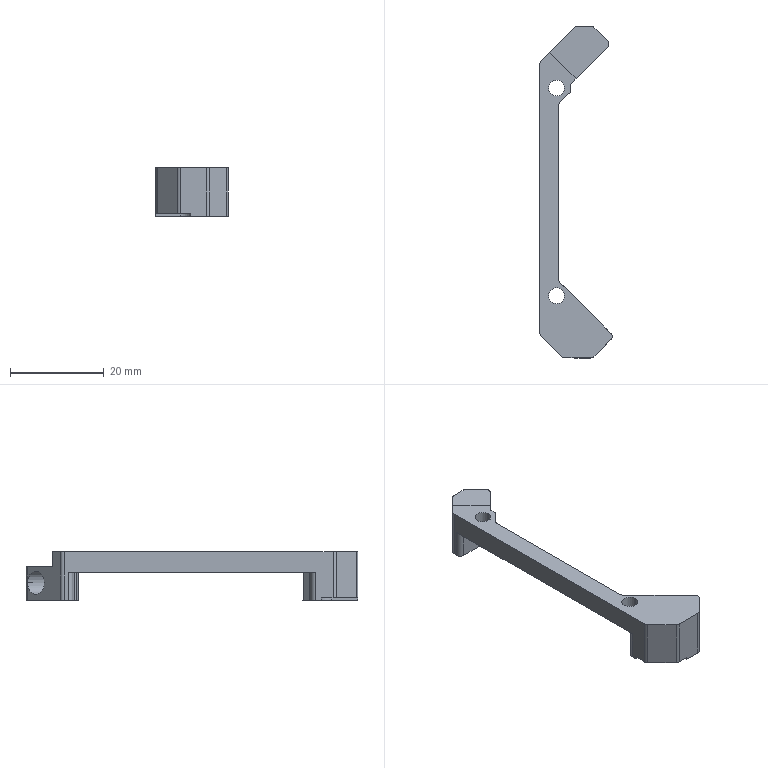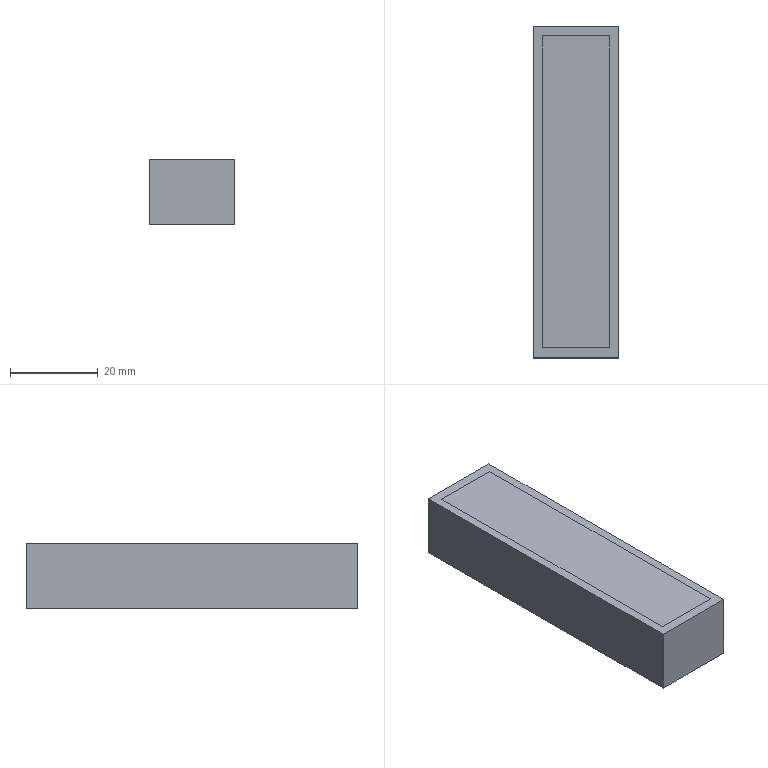CAM job | NX | 3+2 milling, drilling | part box 15.463 x 71 x 10.4 mm | stock box 19.463 x 75.537 x 15 mm
Tools:
number,name,description,diameter,corner_radius,flute_length,length,flutes
5,D4点钻,定心钻D4,4.0,0.0,43.0,75.0,2
3,D2-ROUGHING,D2,2.0,0.0,6.0,50.0,2
11,D3-ROUGHING,D3,3.0,0.0,9.0,50.0,2
7,D4-FINISHING,D4,4.0,0.0,12.0,50.0,2
2,D8-ROUGHING,D8,8.0,0.0,20.0,60.0,2
4,D8-FINISHING,D8,8.0,0.0,20.0,60.0,2
5,D4倒角刀,DJ4-32,4.0,0.0,2.0,50.0,2
1,D54-面刀,Milling Tool-5 Parameters,50.0,0.0,50.0,75.0,2
6,DRILL-3.4,Drilling Tool,3.4,0.0,35.0,50.0,2
10,DRILL-3,Drilling Tool,3.0,0.0,35.0,50.0,2
Operations:
program,operation,operation_type,tool,method,geometry_group,spindle_rpm,surface_speed,feed_per_tooth,feed_cut,feed_plunge,cut_length_mm,path_length_mm,cut_time_min,machine_time_min
G54,FLOOR_FACING,VolumeBased25DMillingOperation,D54-面刀,METHOD,W1,4500.0,706.0,0.0556,500.0,100.0,137.0,231.0,0.274,0.2834
G54,ADAPTIVE_MILLING,CavityMilling,D8-ROUGHING,METHOD,W1,5000.0,125.0,0.3,3000.0,100.0,1565.868,1857.268,0.3669,0.396
G54,PLANAR_MILL_1,PlanarMilling,D2-ROUGHING,METHOD,W1,4000.0,25.0,0.1,800.0,100.0,99.648,254.928,0.1246,0.1401
G54,PLANAR_MILL_1_COPY_1,PlanarMilling,D2-ROUGHING,METHOD,W1,4000.0,25.0,0.1,800.0,100.0,52.68,178.33,0.0658,0.0784
G54,PLANAR_MILL_1_COPY,PlanarMilling,D2-ROUGHING,METHOD,W1,4000.0,25.0,0.0187,150.0,100.0,60.303,257.049,0.402,0.4217
G54,PLANAR_MILL,PlanarMilling,D8-FINISHING,METHOD,W1,5000.0,125.0,0.07,700.0,100.0,424.698,542.698,0.6067,0.6185
G54,PLANAR_MILL_COPY,PlanarMilling,D8-FINISHING,METHOD,W1,5000.0,125.0,0.07,700.0,100.0,48.0,267.682,0.0686,0.0905
G54,PECK_DRILLING,Operation,D4点钻,METHOD,W1,2500.0,18.0,0.05,150.0,0.0,9.4,166.321,0.0627,0.0784
G54,PLANAR_MILL_2,PlanarMilling,D4点钻,METHOD,W1,3000.0,37.0,0.1333,800.0,100.0,169.216,266.216,0.2115,0.2212
G54,PLANAR_MILL_2_COPY,PlanarMilling,D4点钻,METHOD,W1,3000.0,37.0,0.1333,800.0,100.0,37.774,141.274,0.0472,0.0576
G54,PECK_DRILLING_COPY,Operation,DRILL-3.4,METHOD,W1,2500.0,26.0,0.02,100.0,0.0,22.0,191.521,0.22,0.237
G55,FLOOR_FACING_1,VolumeBased25DMillingOperation,D54-面刀,METHOD,W2,4500.0,706.0,0.2222,2000.0,100.0,665.0,1672.4,0.3325,0.4332
G55,FLOOR_FACING_1_COPY,VolumeBased25DMillingOperation,D54-面刀,METHOD,W2,4500.0,706.0,0.0556,500.0,100.0,133.0,237.0,0.266,0.2764
G55,CAVITY_MILL,CavityMilling,D8-ROUGHING,METHOD,W2,5000.0,125.0,0.25,2500.0,100.0,659.673,1089.973,0.2639,0.3069
G55,PLANAR_MILL_3,PlanarMilling,D2-ROUGHING,METHOD,W2,4500.0,28.0,0.1111,1000.0,100.0,156.349,385.613,0.1563,0.1793
G55,PLANAR_MILL_3_COPY,PlanarMilling,D2-ROUGHING,METHOD,W2,4500.0,28.0,0.0333,300.0,100.0,105.891,331.775,0.353,0.3756
G55,PLANAR_MILL_4,PlanarMilling,D8-FINISHING,METHOD,W2,4500.0,113.0,0.0778,700.0,100.0,70.096,317.964,0.1001,0.1249
G55,PLANAR_MILL_4_COPY,PlanarMilling,D8-FINISHING,METHOD,W2,4500.0,113.0,0.0778,700.0,100.0,58.079,164.079,0.083,0.0936
G55,PLANAR_MILL_4_COPY_COPY,PlanarMilling,D4-FINISHING,METHOD,W2,4500.0,56.0,0.1111,1000.0,100.0,31.456,127.456,0.0315,0.0411
G55,PLANAR_MILL_4_COPY_COPY_COPY,PlanarMilling,D4-FINISHING,METHOD,W2,4500.0,56.0,0.0556,500.0,100.0,32.495,128.495,0.065,0.0746
G55,SPOT_DRILLING,Operation,D4倒角刀,METHOD,W2,1500.0,18.0,0.05,150.0,0.0,9.4,69.321,0.0627,0.0687
G55,PLANAR_MILL_5,PlanarMilling,D4倒角刀,METHOD,W2,4500.0,56.0,0.1111,1000.0,100.0,59.426,154.326,0.0594,0.0689
G55,PLANAR_MILL_5_COPY_1,PlanarMilling,D4倒角刀,METHOD,W2,4500.0,56.0,0.1111,1000.0,100.0,20.772,117.772,0.0208,0.0305
G55,PLANAR_MILL_5_COPY,PlanarMilling,D4倒角刀,METHOD,W2,4500.0,56.0,0.1111,1000.0,100.0,57.074,153.073,0.0571,0.0667
G55,PLANAR_MILL_5_COPY_COPY,PlanarMilling,D4倒角刀,METHOD,W2,4500.0,56.0,0.1111,1000.0,100.0,112.25,340.907,0.1123,0.1351
钳口-虎钳,SPOT_DRILLING_1,Operation,D4倒角刀,METHOD,虎钳-钳口,1500.0,18.0,0.05,150.0,0.0,40.5,250.359,0.27,0.291
钳口-虎钳,SPOT_DRILLING_1_COPY,Operation,DRILL-3,METHOD,虎钳-钳口,1500.0,18.0,0.05,150.0,0.0,81.0,331.359,0.54,0.565
钳口-虎钳,FLOOR_WALL,VolumeBased25DMillingOperation,D3-ROUGHING,METHOD,虎钳-钳口,5000.0,47.0,0.2,2000.0,100.0,1956.725,2277.783,0.9784,1.01
钳口-虎钳,FLOOR_WALL_COPY_COPY,VolumeBased25DMillingOperation,D2-ROUGHING,METHOD,虎钳-钳口,5000.0,31.0,0.08,800.0,100.0,341.296,421.147,0.4266,0.4346
钳口-虎钳,FLOOR_WALL_COPY,VolumeBased25DMillingOperation,D2-ROUGHING,METHOD,虎钳-钳口,5000.0,31.0,0.08,800.0,100.0,355.509,401.309,0.4444,0.449
钳口-虎钳,FLOOR_WALL_COPY_COPY_COPY,VolumeBased25DMillingOperation,D2-ROUGHING,METHOD,虎钳-钳口,5000.0,31.0,0.08,800.0,100.0,170.748,211.538,0.2134,0.2175
氧化后加工,FLOOR_WALL_1,VolumeBased25DMillingOperation,D4-FINISHING,METHOD,MCS_3,4000.0,50.0,0.1,800.0,100.0,198.584,325.005,0.2482,0.2609
氧化后加工,PLANAR_MILL_6,PlanarMilling,D4-FINISHING,METHOD,MCS_3,4000.0,50.0,0.025,200.0,100.0,9.712,121.112,0.0486,0.0597
氧化后加工,PLANAR_MILL_6_COPY,PlanarMilling,D4-FINISHING,METHOD,MCS_3,4000.0,50.0,0.025,200.0,100.0,24.74,130.84,0.1237,0.1343
氧化后加工,PLANAR_MILL_7,PlanarMilling,D4点钻,METHOD,MCS_3,3000.0,37.0,0.1167,700.0,100.0,22.336,119.336,0.0319,0.0416
氧化后加工,PLANAR_MILL_7_COPY,PlanarMilling,D4点钻,METHOD,MCS_3,3000.0,37.0,0.1167,700.0,100.0,12.597,121.297,0.018,0.0289
氧化后加工-2,FLOOR_WALL_1_COPY,VolumeBased25DMillingOperation,D4-FINISHING,METHOD,MCS_4,4000.0,50.0,0.05,400.0,100.0,89.648,286.748,0.2241,0.2438
氧化后加工-2,PLANAR_MILL_6_COPY_1,PlanarMilling,D4-FINISHING,METHOD,MCS_4,4000.0,50.0,0.01,80.0,100.0,19.231,131.731,0.2404,0.2516
氧化后加工-2,PLANAR_MILL_8,PlanarMilling,D4倒角刀,METHOD,MCS_4,3500.0,43.0,0.0286,200.0,100.0,15.582,112.582,0.0779,0.0876